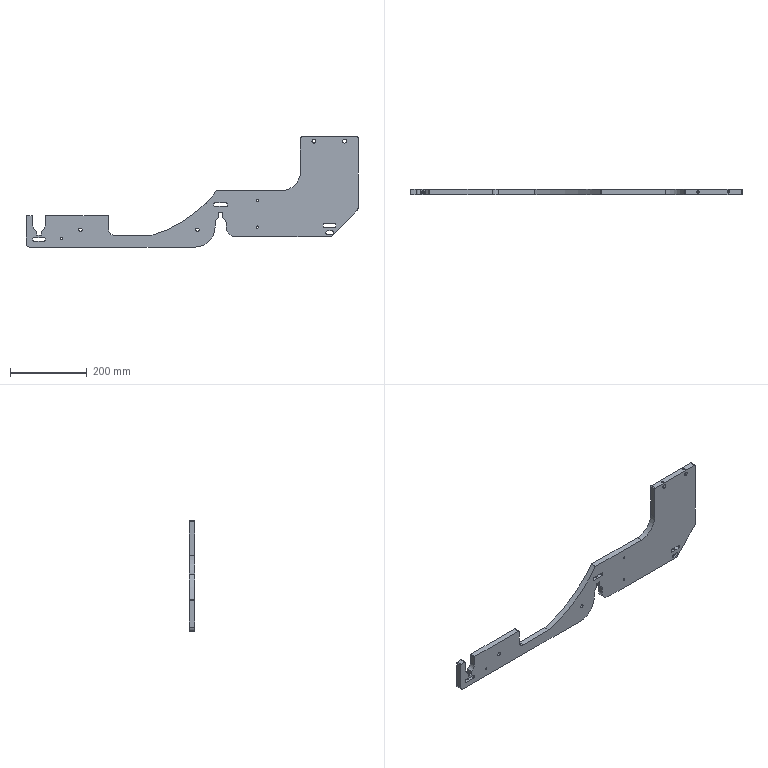Part | STEP file | Right | 1 solid | 138 faces | box 866 x 15 x 287 mm | volume 1373822 mm3 | plane 60 | cylinder 53 | other 20 | cone 5 | commonest cylinder face diameters 4 x15 6 x10 8 x5 5 x4 10 x4 9 x2